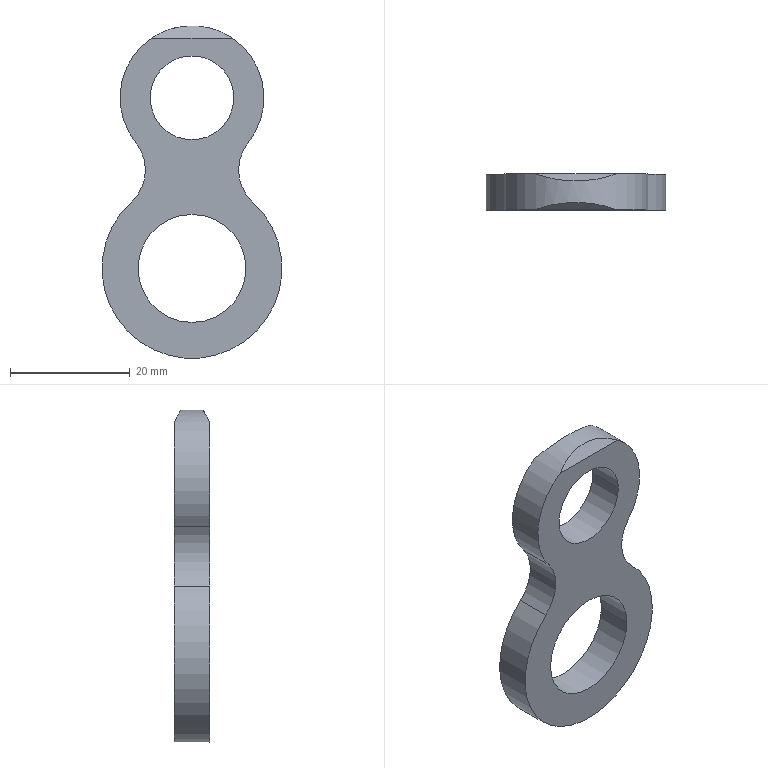Part | NX | features BREP 1 | 1 solid | 12 faces | box 30 x 6 x 55.457 mm | volume 4802 mm3 | cylinder 8 | plane 4 | commonest cylinder face diameters 14 x2 14.472 x2 18 x2 24 x1 30 x1
STEP:
#1=CARTESIAN_POINT('',(-10.119,3.,11.073));
#2=VERTEX_POINT('',#1);
#3=CARTESIAN_POINT('',(10.119,3.,11.073));
#4=VERTEX_POINT('',#3);
#5=CARTESIAN_POINT('',(0.,3.,0.));
#6=DIRECTION('',(0.,-1.,0.));
#7=DIRECTION('',(-0.6746,0.,0.7382));
#8=AXIS2_PLACEMENT_3D('',#5,#6,#7);
#9=CIRCLE('',#8,15.);
#10=EDGE_CURVE('',#2,#4,#9,.T.);
#11=ORIENTED_EDGE('',*,*,#10,.T.);
#12=CARTESIAN_POINT('',(10.119,-3.,11.073));
#13=VERTEX_POINT('',#12);
#14=CARTESIAN_POINT('',(10.119,-3.,11.073));
#15=DIRECTION('',(0.,1.,0.));
#16=VECTOR('',#15,1000.);
#17=LINE('',#14,#16);
#18=EDGE_CURVE('',#13,#4,#17,.T.);
#19=ORIENTED_EDGE('',*,*,#18,.F.);
#20=CARTESIAN_POINT('',(-10.119,-3.,11.073));
#21=VERTEX_POINT('',#20);
#22=CARTESIAN_POINT('',(0.,-3.,0.));
#23=DIRECTION('',(0.,-1.,0.));
#24=DIRECTION('',(-0.6746,0.,0.7382));
#25=AXIS2_PLACEMENT_3D('',#22,#23,#24);
#26=CIRCLE('',#25,15.);
#27=EDGE_CURVE('',#21,#13,#26,.T.);
#28=ORIENTED_EDGE('',*,*,#27,.F.);
#29=CARTESIAN_POINT('',(-10.119,-3.,11.073));
#30=DIRECTION('',(0.,1.,0.));
#31=VECTOR('',#30,1000.);
#32=LINE('',#29,#31);
#33=EDGE_CURVE('',#21,#2,#32,.T.);
#34=ORIENTED_EDGE('',*,*,#33,.T.);
#35=EDGE_LOOP('',(#11,#19,#28,#34));
#36=FACE_BOUND('',#35,.T.);
#37=CARTESIAN_POINT('',(0.,3.,0.));
#38=DIRECTION('',(0.,-1.,0.));
#39=DIRECTION('',(0.,0.,-1.));
#40=AXIS2_PLACEMENT_3D('',#37,#38,#39);
#41=CYLINDRICAL_SURFACE('',#40,15.);
#42=ADVANCED_FACE('',(#36),#41,.T.);
#43=ORIENTED_EDGE('',*,*,#18,.T.);
#44=CARTESIAN_POINT('',(9.357,3.,20.945));
#45=VERTEX_POINT('',#44);
#46=CARTESIAN_POINT('',(15.,3.,16.415));
#47=DIRECTION('',(0.,1.,0.));
#48=DIRECTION('',(-0.6746,0.,-0.7382));
#49=AXIS2_PLACEMENT_3D('',#46,#47,#48);
#50=CIRCLE('',#49,7.236);
#51=EDGE_CURVE('',#4,#45,#50,.T.);
#52=ORIENTED_EDGE('',*,*,#51,.T.);
#53=CARTESIAN_POINT('',(9.357,-3.,20.945));
#54=VERTEX_POINT('',#53);
#55=CARTESIAN_POINT('',(9.357,-3.,20.945));
#56=DIRECTION('',(0.,1.,0.));
#57=VECTOR('',#56,1000.);
#58=LINE('',#55,#57);
#59=EDGE_CURVE('',#54,#45,#58,.T.);
#60=ORIENTED_EDGE('',*,*,#59,.F.);
#61=CARTESIAN_POINT('',(15.,-3.,16.415));
#62=DIRECTION('',(0.,1.,0.));
#63=DIRECTION('',(-0.6746,0.,-0.7382));
#64=AXIS2_PLACEMENT_3D('',#61,#62,#63);
#65=CIRCLE('',#64,7.236);
#66=EDGE_CURVE('',#13,#54,#65,.T.);
#67=ORIENTED_EDGE('',*,*,#66,.F.);
#68=EDGE_LOOP('',(#43,#52,#60,#67));
#69=FACE_BOUND('',#68,.T.);
#70=CARTESIAN_POINT('',(15.,3.,16.415));
#71=DIRECTION('',(0.,-1.,0.));
#72=DIRECTION('',(-0.997,0.,-0.07689));
#73=AXIS2_PLACEMENT_3D('',#70,#71,#72);
#74=CYLINDRICAL_SURFACE('',#73,7.236);
#75=ADVANCED_FACE('',(#69),#74,.F.);
#76=CARTESIAN_POINT('',(-9.357,-3.,20.945));
#77=VERTEX_POINT('',#76);
#78=CARTESIAN_POINT('',(-9.357,3.,20.945));
#79=VERTEX_POINT('',#78);
#80=CARTESIAN_POINT('',(-9.357,-3.,20.945));
#81=DIRECTION('',(0.,1.,0.));
#82=VECTOR('',#81,1000.);
#83=LINE('',#80,#82);
#84=EDGE_CURVE('',#77,#79,#83,.T.);
#85=ORIENTED_EDGE('',*,*,#84,.T.);
#86=CARTESIAN_POINT('',(-15.,3.,16.415));
#87=DIRECTION('',(0.,1.,0.));
#88=DIRECTION('',(0.7798,0.,0.626));
#89=AXIS2_PLACEMENT_3D('',#86,#87,#88);
#90=CIRCLE('',#89,7.236);
#91=EDGE_CURVE('',#79,#2,#90,.T.);
#92=ORIENTED_EDGE('',*,*,#91,.T.);
#93=ORIENTED_EDGE('',*,*,#33,.F.);
#94=CARTESIAN_POINT('',(-15.,-3.,16.415));
#95=DIRECTION('',(0.,1.,0.));
#96=DIRECTION('',(0.7798,0.,0.626));
#97=AXIS2_PLACEMENT_3D('',#94,#95,#96);
#98=CIRCLE('',#97,7.236);
#99=EDGE_CURVE('',#77,#21,#98,.T.);
#100=ORIENTED_EDGE('',*,*,#99,.F.);
#101=EDGE_LOOP('',(#85,#92,#93,#100));
#102=FACE_BOUND('',#101,.T.);
#103=CARTESIAN_POINT('',(-15.,3.,16.415));
#104=DIRECTION('',(0.,-1.,0.));
#105=DIRECTION('',(0.997,0.,-0.07689));
#106=AXIS2_PLACEMENT_3D('',#103,#104,#105);
#107=CYLINDRICAL_SURFACE('',#106,7.236);
#108=ADVANCED_FACE('',(#102),#107,.F.);
#109=CARTESIAN_POINT('',(9.,3.,0.));
#110=VERTEX_POINT('',#109);
#111=CARTESIAN_POINT('',(9.,-3.,0.));
#112=VERTEX_POINT('',#111);
#113=CARTESIAN_POINT('',(9.,-3.,0.));
#114=DIRECTION('',(0.,1.,0.));
#115=VECTOR('',#114,1000.);
#116=LINE('',#113,#115);
#117=EDGE_CURVE('',#110,#112,#116,.F.);
#118=ORIENTED_EDGE('',*,*,#117,.F.);
#119=CARTESIAN_POINT('',(-9.,3.,0.));
#120=VERTEX_POINT('',#119);
#121=CARTESIAN_POINT('',(0.,3.,0.));
#122=DIRECTION('',(0.,-1.,0.));
#123=DIRECTION('',(-1.,0.,0.));
#124=AXIS2_PLACEMENT_3D('',#121,#122,#123);
#125=CIRCLE('',#124,9.);
#126=EDGE_CURVE('',#120,#110,#125,.T.);
#127=ORIENTED_EDGE('',*,*,#126,.F.);
#128=CARTESIAN_POINT('',(-9.,-3.,0.));
#129=VERTEX_POINT('',#128);
#130=CARTESIAN_POINT('',(-9.,-3.,0.));
#131=DIRECTION('',(0.,1.,0.));
#132=VECTOR('',#131,1000.);
#133=LINE('',#130,#132);
#134=EDGE_CURVE('',#120,#129,#133,.F.);
#135=ORIENTED_EDGE('',*,*,#134,.T.);
#136=CARTESIAN_POINT('',(0.,-3.,0.));
#137=DIRECTION('',(0.,-1.,0.));
#138=DIRECTION('',(-1.,0.,0.));
#139=AXIS2_PLACEMENT_3D('',#136,#137,#138);
#140=CIRCLE('',#139,9.);
#141=EDGE_CURVE('',#129,#112,#140,.T.);
#142=ORIENTED_EDGE('',*,*,#141,.T.);
#143=EDGE_LOOP('',(#118,#127,#135,#142));
#144=FACE_BOUND('',#143,.T.);
#145=CARTESIAN_POINT('',(0.,3.,0.));
#146=DIRECTION('',(0.,-1.,0.));
#147=DIRECTION('',(-1.,0.,0.));
#148=AXIS2_PLACEMENT_3D('',#145,#146,#147);
#149=CYLINDRICAL_SURFACE('',#148,9.);
#150=ADVANCED_FACE('',(#144),#149,.F.);
#151=CARTESIAN_POINT('',(0.,3.,0.));
#152=DIRECTION('',(0.,-1.,0.));
#153=DIRECTION('',(1.,0.,0.));
#154=AXIS2_PLACEMENT_3D('',#151,#152,#153);
#155=CIRCLE('',#154,9.);
#156=EDGE_CURVE('',#110,#120,#155,.T.);
#157=ORIENTED_EDGE('',*,*,#156,.F.);
#158=ORIENTED_EDGE('',*,*,#117,.T.);
#159=CARTESIAN_POINT('',(0.,-3.,0.));
#160=DIRECTION('',(0.,-1.,0.));
#161=DIRECTION('',(1.,0.,0.));
#162=AXIS2_PLACEMENT_3D('',#159,#160,#161);
#163=CIRCLE('',#162,9.);
#164=EDGE_CURVE('',#112,#129,#163,.T.);
#165=ORIENTED_EDGE('',*,*,#164,.T.);
#166=ORIENTED_EDGE('',*,*,#134,.F.);
#167=EDGE_LOOP('',(#157,#158,#165,#166));
#168=FACE_BOUND('',#167,.T.);
#169=CARTESIAN_POINT('',(0.,3.,0.));
#170=DIRECTION('',(0.,-1.,0.));
#171=DIRECTION('',(-1.,0.,0.));
#172=AXIS2_PLACEMENT_3D('',#169,#170,#171);
#173=CYLINDRICAL_SURFACE('',#172,9.);
#174=ADVANCED_FACE('',(#168),#173,.F.);
#175=CARTESIAN_POINT('',(7.,3.,28.457));
#176=VERTEX_POINT('',#175);
#177=CARTESIAN_POINT('',(7.,-3.,28.457));
#178=VERTEX_POINT('',#177);
#179=CARTESIAN_POINT('',(7.,-3.,28.457));
#180=DIRECTION('',(0.,1.,0.));
#181=VECTOR('',#180,1000.);
#182=LINE('',#179,#181);
#183=EDGE_CURVE('',#176,#178,#182,.F.);
#184=ORIENTED_EDGE('',*,*,#183,.F.);
#185=CARTESIAN_POINT('',(-7.,3.,28.457));
#186=VERTEX_POINT('',#185);
#187=CARTESIAN_POINT('',(0.,3.,28.457));
#188=DIRECTION('',(0.,-1.,0.));
#189=DIRECTION('',(-1.,0.,0.));
#190=AXIS2_PLACEMENT_3D('',#187,#188,#189);
#191=CIRCLE('',#190,7.);
#192=EDGE_CURVE('',#186,#176,#191,.T.);
#193=ORIENTED_EDGE('',*,*,#192,.F.);
#194=CARTESIAN_POINT('',(-7.,-3.,28.457));
#195=VERTEX_POINT('',#194);
#196=CARTESIAN_POINT('',(-7.,-3.,28.457));
#197=DIRECTION('',(0.,1.,0.));
#198=VECTOR('',#197,1000.);
#199=LINE('',#196,#198);
#200=EDGE_CURVE('',#186,#195,#199,.F.);
#201=ORIENTED_EDGE('',*,*,#200,.T.);
#202=CARTESIAN_POINT('',(0.,-3.,28.457));
#203=DIRECTION('',(0.,-1.,0.));
#204=DIRECTION('',(-1.,0.,0.));
#205=AXIS2_PLACEMENT_3D('',#202,#203,#204);
#206=CIRCLE('',#205,7.);
#207=EDGE_CURVE('',#195,#178,#206,.T.);
#208=ORIENTED_EDGE('',*,*,#207,.T.);
#209=EDGE_LOOP('',(#184,#193,#201,#208));
#210=FACE_BOUND('',#209,.T.);
#211=CARTESIAN_POINT('',(0.,3.,28.457));
#212=DIRECTION('',(0.,-1.,0.));
#213=DIRECTION('',(-1.,0.,0.));
#214=AXIS2_PLACEMENT_3D('',#211,#212,#213);
#215=CYLINDRICAL_SURFACE('',#214,7.);
#216=ADVANCED_FACE('',(#210),#215,.F.);
#217=CARTESIAN_POINT('',(0.,3.,28.457));
#218=DIRECTION('',(0.,-1.,0.));
#219=DIRECTION('',(1.,0.,0.));
#220=AXIS2_PLACEMENT_3D('',#217,#218,#219);
#221=CIRCLE('',#220,7.);
#222=EDGE_CURVE('',#176,#186,#221,.T.);
#223=ORIENTED_EDGE('',*,*,#222,.F.);
#224=ORIENTED_EDGE('',*,*,#183,.T.);
#225=CARTESIAN_POINT('',(0.,-3.,28.457));
#226=DIRECTION('',(0.,-1.,0.));
#227=DIRECTION('',(1.,0.,0.));
#228=AXIS2_PLACEMENT_3D('',#225,#226,#227);
#229=CIRCLE('',#228,7.);
#230=EDGE_CURVE('',#178,#195,#229,.T.);
#231=ORIENTED_EDGE('',*,*,#230,.T.);
#232=ORIENTED_EDGE('',*,*,#200,.F.);
#233=EDGE_LOOP('',(#223,#224,#231,#232));
#234=FACE_BOUND('',#233,.T.);
#235=CARTESIAN_POINT('',(0.,3.,28.457));
#236=DIRECTION('',(0.,-1.,0.));
#237=DIRECTION('',(-1.,0.,0.));
#238=AXIS2_PLACEMENT_3D('',#235,#236,#237);
#239=CYLINDRICAL_SURFACE('',#238,7.);
#240=ADVANCED_FACE('',(#234),#239,.F.);
#241=CARTESIAN_POINT('',(-6.75,3.,38.379));
#242=VERTEX_POINT('',#241);
#243=CARTESIAN_POINT('',(0.,3.,28.457));
#244=DIRECTION('',(0.,-1.,0.));
#245=DIRECTION('',(-0.5625,0.,0.8268));
#246=AXIS2_PLACEMENT_3D('',#243,#244,#245);
#247=CIRCLE('',#246,12.);
#248=EDGE_CURVE('',#242,#79,#247,.T.);
#249=ORIENTED_EDGE('',*,*,#248,.F.);
#250=CARTESIAN_POINT('',(6.75,3.,38.379));
#251=VERTEX_POINT('',#250);
#252=CARTESIAN_POINT('',(-6.75,3.,38.379));
#253=DIRECTION('',(1.,0.,0.));
#254=VECTOR('',#253,1000.);
#255=LINE('',#252,#254);
#256=EDGE_CURVE('',#242,#251,#255,.T.);
#257=ORIENTED_EDGE('',*,*,#256,.T.);
#258=CARTESIAN_POINT('',(0.,3.,28.457));
#259=DIRECTION('',(0.,-1.,0.));
#260=DIRECTION('',(0.7798,0.,-0.626));
#261=AXIS2_PLACEMENT_3D('',#258,#259,#260);
#262=CIRCLE('',#261,12.);
#263=EDGE_CURVE('',#45,#251,#262,.T.);
#264=ORIENTED_EDGE('',*,*,#263,.F.);
#265=ORIENTED_EDGE('',*,*,#51,.F.);
#266=ORIENTED_EDGE('',*,*,#10,.F.);
#267=ORIENTED_EDGE('',*,*,#91,.F.);
#268=EDGE_LOOP('',(#249,#257,#264,#265,#266,#267));
#269=FACE_BOUND('',#268,.T.);
#270=ORIENTED_EDGE('',*,*,#126,.T.);
#271=ORIENTED_EDGE('',*,*,#156,.T.);
#272=EDGE_LOOP('',(#270,#271));
#273=FACE_BOUND('',#272,.T.);
#274=ORIENTED_EDGE('',*,*,#192,.T.);
#275=ORIENTED_EDGE('',*,*,#222,.T.);
#276=EDGE_LOOP('',(#274,#275));
#277=FACE_BOUND('',#276,.T.);
#278=CARTESIAN_POINT('',(-46.381,3.,-43.125));
#279=DIRECTION('',(0.,1.,0.));
#280=DIRECTION('',(-1.,0.,0.));
#281=AXIS2_PLACEMENT_3D('',#278,#279,#280);
#282=PLANE('',#281);
#283=ADVANCED_FACE('',(#269,#273,#277),#282,.T.);
#284=CARTESIAN_POINT('',(-6.75,-3.,38.379));
#285=VERTEX_POINT('',#284);
#286=CARTESIAN_POINT('',(0.,-3.,28.457));
#287=DIRECTION('',(0.,-1.,0.));
#288=DIRECTION('',(-0.5625,0.,0.8268));
#289=AXIS2_PLACEMENT_3D('',#286,#287,#288);
#290=CIRCLE('',#289,12.);
#291=EDGE_CURVE('',#285,#77,#290,.T.);
#292=ORIENTED_EDGE('',*,*,#291,.T.);
#293=ORIENTED_EDGE('',*,*,#99,.T.);
#294=ORIENTED_EDGE('',*,*,#27,.T.);
#295=ORIENTED_EDGE('',*,*,#66,.T.);
#296=CARTESIAN_POINT('',(6.75,-3.,38.379));
#297=VERTEX_POINT('',#296);
#298=CARTESIAN_POINT('',(0.,-3.,28.457));
#299=DIRECTION('',(0.,-1.,0.));
#300=DIRECTION('',(0.7798,0.,-0.626));
#301=AXIS2_PLACEMENT_3D('',#298,#299,#300);
#302=CIRCLE('',#301,12.);
#303=EDGE_CURVE('',#54,#297,#302,.T.);
#304=ORIENTED_EDGE('',*,*,#303,.T.);
#305=CARTESIAN_POINT('',(-6.75,-3.,38.379));
#306=DIRECTION('',(1.,0.,0.));
#307=VECTOR('',#306,1000.);
#308=LINE('',#305,#307);
#309=EDGE_CURVE('',#285,#297,#308,.T.);
#310=ORIENTED_EDGE('',*,*,#309,.F.);
#311=EDGE_LOOP('',(#292,#293,#294,#295,#304,#310));
#312=FACE_BOUND('',#311,.T.);
#313=ORIENTED_EDGE('',*,*,#141,.F.);
#314=ORIENTED_EDGE('',*,*,#164,.F.);
#315=EDGE_LOOP('',(#313,#314));
#316=FACE_BOUND('',#315,.T.);
#317=ORIENTED_EDGE('',*,*,#207,.F.);
#318=ORIENTED_EDGE('',*,*,#230,.F.);
#319=EDGE_LOOP('',(#317,#318));
#320=FACE_BOUND('',#319,.T.);
#321=CARTESIAN_POINT('',(-46.381,-3.,-43.125));
#322=DIRECTION('',(0.,-1.,0.));
#323=DIRECTION('',(0.,0.,1.));
#324=AXIS2_PLACEMENT_3D('',#321,#322,#323);
#325=PLANE('',#324);
#326=ADVANCED_FACE('',(#312,#316,#320),#325,.T.);
#327=ORIENTED_EDGE('',*,*,#248,.T.);
#328=ORIENTED_EDGE('',*,*,#84,.F.);
#329=ORIENTED_EDGE('',*,*,#291,.F.);
#330=CARTESIAN_POINT('',(0.,-8.728,28.457));
#331=DIRECTION('',(0.,-0.866,0.5));
#332=DIRECTION('',(0.,-0.5,-0.866));
#333=AXIS2_PLACEMENT_3D('',#330,#331,#332);
#334=ELLIPSE('',#333,13.856,12.);
#335=EDGE_CURVE('',#297,#285,#334,.T.);
#336=ORIENTED_EDGE('',*,*,#335,.F.);
#337=ORIENTED_EDGE('',*,*,#303,.F.);
#338=ORIENTED_EDGE('',*,*,#59,.T.);
#339=ORIENTED_EDGE('',*,*,#263,.T.);
#340=CARTESIAN_POINT('',(0.,8.728,28.457));
#341=DIRECTION('',(0.,0.866,0.5));
#342=DIRECTION('',(0.,-0.5,0.866));
#343=AXIS2_PLACEMENT_3D('',#340,#341,#342);
#344=ELLIPSE('',#343,13.856,12.);
#345=EDGE_CURVE('',#242,#251,#344,.T.);
#346=ORIENTED_EDGE('',*,*,#345,.F.);
#347=EDGE_LOOP('',(#327,#328,#329,#336,#337,#338,#339,#346));
#348=FACE_BOUND('',#347,.T.);
#349=CARTESIAN_POINT('',(0.,3.,28.457));
#350=DIRECTION('',(0.,-1.,0.));
#351=DIRECTION('',(0.,0.,1.));
#352=AXIS2_PLACEMENT_3D('',#349,#350,#351);
#353=CYLINDRICAL_SURFACE('',#352,12.);
#354=ADVANCED_FACE('',(#348),#353,.T.);
#355=ORIENTED_EDGE('',*,*,#256,.F.);
#356=ORIENTED_EDGE('',*,*,#345,.T.);
#357=EDGE_LOOP('',(#355,#356));
#358=FACE_BOUND('',#357,.T.);
#359=CARTESIAN_POINT('',(6.75,1.706,40.62));
#360=DIRECTION('',(0.,0.866,0.5));
#361=DIRECTION('',(-1.,0.,0.));
#362=AXIS2_PLACEMENT_3D('',#359,#360,#361);
#363=PLANE('',#362);
#364=ADVANCED_FACE('',(#358),#363,.T.);
#365=ORIENTED_EDGE('',*,*,#335,.T.);
#366=ORIENTED_EDGE('',*,*,#309,.T.);
#367=EDGE_LOOP('',(#365,#366));
#368=FACE_BOUND('',#367,.T.);
#369=CARTESIAN_POINT('',(6.75,-1.706,40.62));
#370=DIRECTION('',(0.,-0.866,0.5));
#371=DIRECTION('',(1.,0.,0.));
#372=AXIS2_PLACEMENT_3D('',#369,#370,#371);
#373=PLANE('',#372);
#374=ADVANCED_FACE('',(#368),#373,.T.);
#375=CLOSED_SHELL('',(#42,#75,#108,#150,#174,#216,#240,#283,#326,#354,#364,#374));
#376=MANIFOLD_SOLID_BREP('',#375);
#377=(LENGTH_UNIT()NAMED_UNIT(*)SI_UNIT(.MILLI.,.METRE.));
#378=UNCERTAINTY_MEASURE_WITH_UNIT(LENGTH_MEASURE(0.00001),#377,'','');
#379=(NAMED_UNIT(*)PLANE_ANGLE_UNIT()SI_UNIT($,.RADIAN.));
#380=(NAMED_UNIT(*)SI_UNIT($,.STERADIAN.)SOLID_ANGLE_UNIT());
#381=(GEOMETRIC_REPRESENTATION_CONTEXT(3)GLOBAL_UNCERTAINTY_ASSIGNED_CONTEXT((#378))GLOBAL_UNIT_ASSIGNED_CONTEXT((#377,#379,#380))REPRESENTATION_CONTEXT('',''));
#382=ADVANCED_BREP_SHAPE_REPRESENTATION('',(#376),#381);